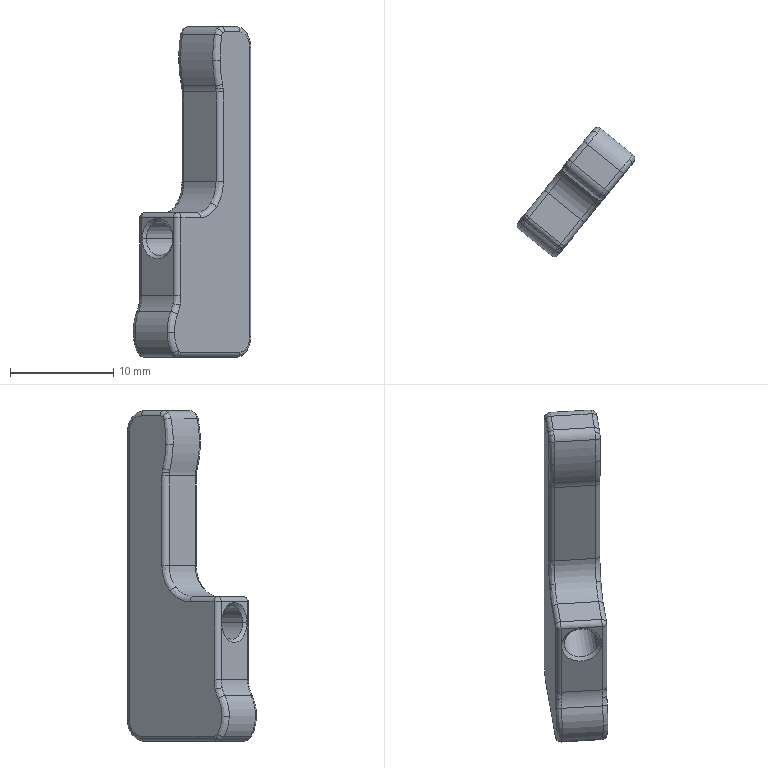Part | SolidWorks | features BaseBody 1 | 1 solid | 75 faces | box 11.394 x 12.489 x 32 mm | volume 1183 mm3 | spline 38 | cylinder 25 | plane 8 | cone 4 | commonest cylinder face diameters 1 x14 4 x3 2 x2 3.3 x2 6 x2 7.248 x1